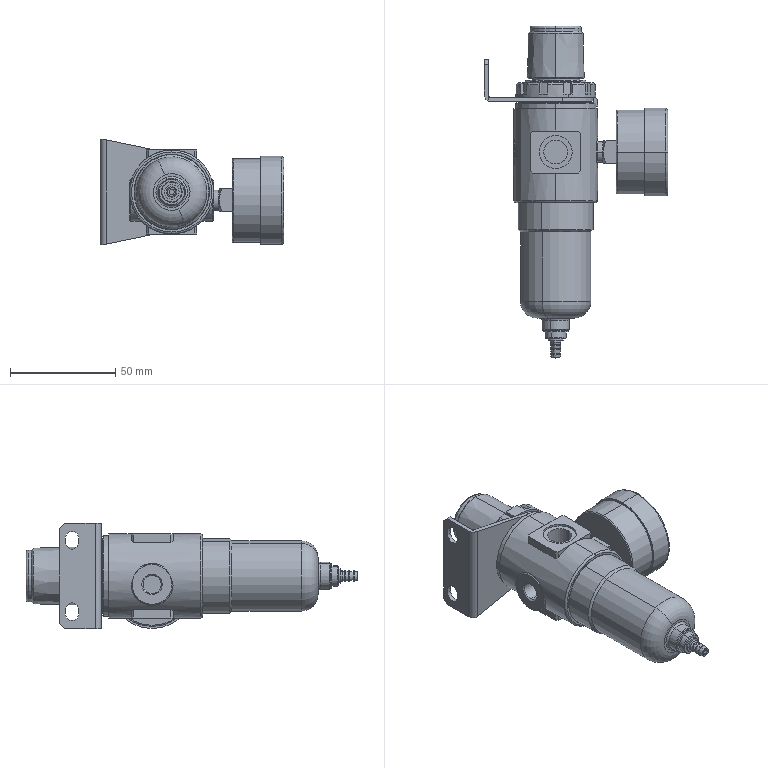Part | SolidWorks | features AEMSimFeature 1 | 5 solids | 277 faces | box 87.334 x 158 x 50 mm | volume 129441 mm3 | plane 112 | cylinder 95 | cone 52 | torus 14 | spline 4 | commonest cylinder face diameters 35.2 x10 5 x8 13 x6 6.4 x4 8.566 x4 11.445 x4